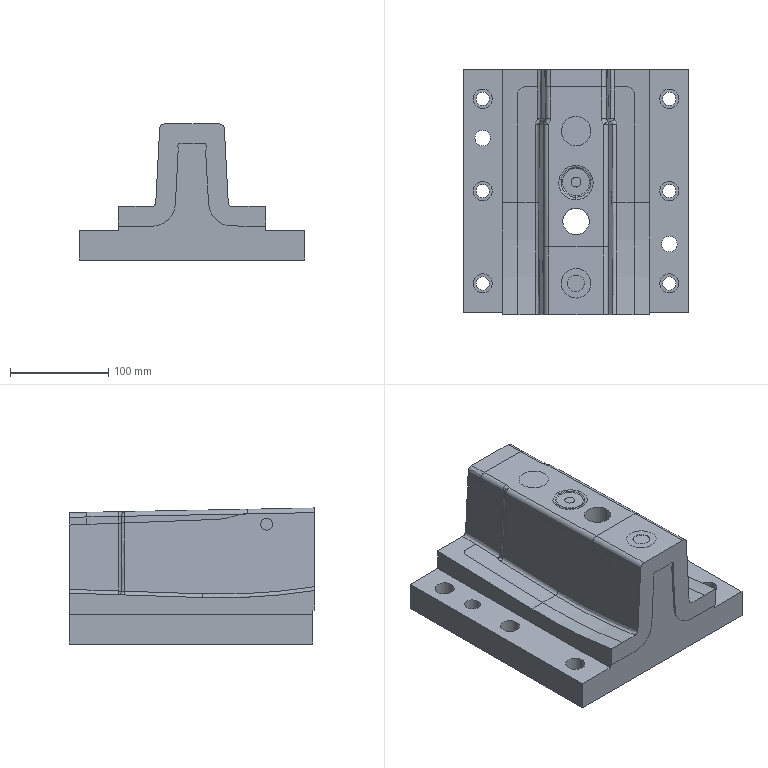Part | NX | features solid 2 | 1 solid | 102 faces | box 230 x 250 x 138.496 mm | volume 3801752 mm3 | spline 50 | plane 26 | cylinder 24 | sphere 2 | commonest cylinder face diameters 10 x8 13.5 x6 19.5 x6 16 x2 17 x1 27 x1